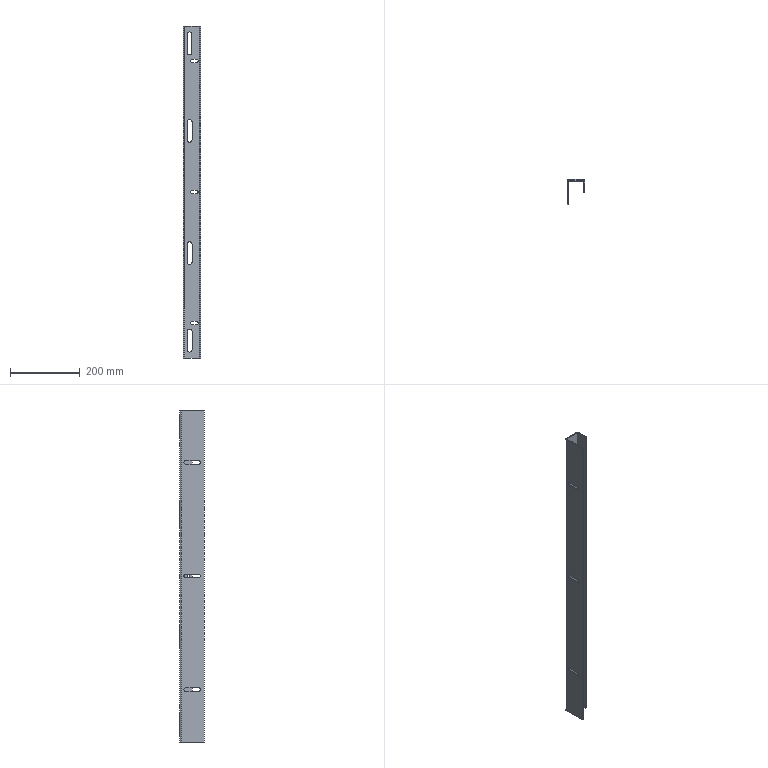Part | SolidWorks | features ICE 3, FlatPattern 1, SMBaseFlange 1, SheetMetal 1 | 1 solid | 71 faces | box 50 x 70 x 950 mm | volume 401871 mm3 | plane 38 | cylinder 33 | commonest cylinder face diameters 10 x15 14 x8 7 x6 2 x2 8 x2